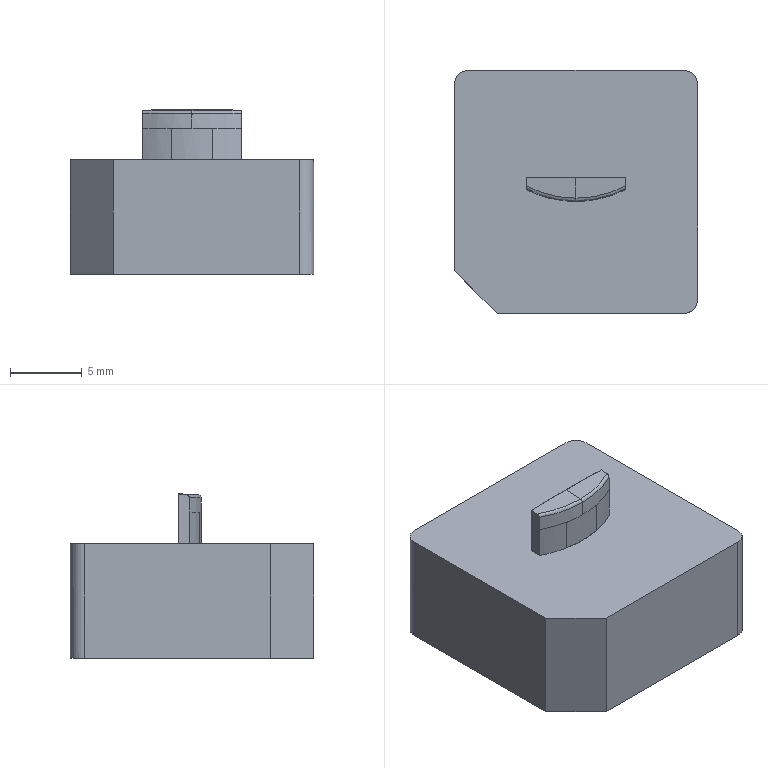NC program | PowerMill | posted with a generic post | part box 17 x 17 x 11.498 mm
Lines 1 to 991 of 31087:
%
O0001
N104 ( POWERMILL CB  : 2026004.0)
N105 ( POST VER      : 2026.0.0.5161)
N106 ( OPTION FILE   : FANUC)
N107 ( OUTPUT WORKPLANE : WORLD)
N108 (  )
N109 ( TOOL LIST )
N110 (-------------------------------------)
N111 ( NO. | ID      | DIA.| TIP RAD|LENGTH)
N112 (-------------------------------------)
N113 (    1|D10C_1_1 |10.0 |  0.0   |66.96 )
N114 (    2|D4C_1    | 4.0 |  0.0   | 59.0 )
N115 (    3|D10_1_1  |10.0 |  0.0   |66.64 )
N116 (    4|R1_1     | 2.0 |  1.0   | 57.0 )
N117 (   10|D3_1_1   | 3.0 |  0.0   |58.76 )
N118 (   13|TEXT_D4_1| 4.0 |  0.3   | 60.0 )
N119 (-------------------------------------)
N120 (  )
N121 ( NUMBER OF TOOLPATHS: 9.0 )
N122 ( ESTIMATED PROGRAM DURATION: 0 HOURS 2 MIN 53 SEC)
N123 (  )
N124 G00 G21 G80 G40 G17
N125 G90
N126 G54
N127 G53 Z0.0
N128 (---------------)
N129 ( START TOOLPATH : 精公开粗01-扫面平行-D10C )
N130 (---------------)
N131 ( TOOL NO.    :1 )
N132 ( TOOL TYPE   : ENDMILL)
N133 ( TOOL ID     : D10C_1_1)
N134 ( TOOL DIA    : 10.0 LENGTH 66.96)
N135 T1
N136 M6
N137 S8000 M03
N138 G00 G90 X0.0 Y0.0
N139 G43 Z10.2 H1
N140
N141 G05 P10000 R4
N142 X11.28 Y11.28
N143 Z1.128
N144 G01 Z-0.072 F6000.0
N145 X-11.28 F10000.0
N146 Y5.64
N147 X11.28
N148 Y0.0
N149 X-11.28
N150 Y-5.64
N151 X11.28
N152 Y-11.28
N153 X-11.28
N154 X-16.28
N155 G00 Z10.2
N156 G05 P0
N157 (---------------)
N158 ( END TOOLPATH : 精公开粗01-扫面平行-D10C )
N159 (---------------)
N160 ( START TOOLPATH : 精公开粗01-外形偏置-D10C )
N161 (---------------)
N162 G00 X0.0 Y0.0 Z9.878
N163 G05 P10000 R4
N164 X16.555 Y5.9194
N165 Z0.7016
N166 G01 Z-0.4984 F6000.0
N167 X16.0275 F10000.0
N168 G03 X11.28 Y1.1719 I0.0 J-4.7475
N169 G01 Y-10.28
N170 G02 X10.28 Y-11.28 I-1.0 J0.0
N171 G01 X-10.28
N172 G02 X-11.28 Y-10.28 I0.0 J1.0
N173 G01 Y10.28
N174 G02 X-10.28 Y11.28 I1.0 J0.0
N175 G01 X10.28
N176 G02 X11.28 Y10.28 I0.0 J-1.0
N177 G01 Y1.1719
N178 X8.7307 Y1.1601
N179 X8.7343 Y0.3867
N180 X8.7011 Y-0.3867
N181 X8.5538 Y-1.1601
N182 X8.2859 Y-1.9336
N183 X8.121 Y-2.2752
N184 X7.8634 Y-2.707
N185 X7.3476 Y-3.3716
N186 X6.5741 Y-4.0652
N187 X6.299 Y-4.2538
N188 X5.8007 Y-4.5354
N189 X4.6946 Y-5.0273
N190 X3.4804 Y-5.4313
N191 X2.707 Y-5.6154
N192 X1.6745 Y-5.8007
N193 X0.3867 Y-5.9046
N194 X-0.3867
N195 X-1.6743 Y-5.8007
N196 X-2.707 Y-5.6173
N197 X-3.4804 Y-5.4312
N198 X-4.2538 Y-5.1896
N199 X-4.6933 Y-5.0273
N200 X-5.8007 Y-4.5354
N201 X-6.3008 Y-4.2538
N202 X-6.5741 Y-4.0652
N203 X-7.2448 Y-3.4804
N204 X-7.8635 Y-2.707
N205 X-8.121 Y-2.2752
N206 X-8.2861 Y-1.9336
N207 X-8.5541 Y-1.1601
N208 X-8.6996 Y-0.3867
N209 X-8.7343 Y0.3867
N210 X-8.7307 Y1.1601
N211 X-8.6458 Y1.9336
N212 X-8.441 Y2.707
N213 X-8.121 Y3.442
N214 X-7.5905 Y4.2538
N215 X-7.3476 Y4.5389
N216 X-6.836 Y5.0273
N217 X-6.5741 Y5.232
N218 X-5.8007 Y5.7023
N219 X-5.0273 Y6.0126
N220 X-4.2538 Y6.1915
N221 X-3.4804 Y6.2524
N222 X3.4804
N223 X4.2538 Y6.1916
N224 X5.0273 Y6.0126
N225 X5.8007 Y5.7023
N226 X6.5741 Y5.232
N227 X6.836 Y5.0273
N228 X7.3476 Y4.5389
N229 X7.5906 Y4.2538
N230 X8.1004 Y3.4804
N231 X8.441 Y2.707
N232 X8.6459 Y1.9336
N233 X8.7307 Y1.1601
N234 X11.28 Y1.1719
N235 G00 Z3.3251
N236 G01 X16.555 Y5.9194
N237 G00 Z0.3251
N238 G01 Z-0.8749 F6000.0
N239 X16.0275 F10000.0
N240 G03 X11.28 Y1.1719 I0.0 J-4.7475
N241 G01 Y-10.28
N242 G02 X10.28 Y-11.28 I-1.0 J0.0
N243 G01 X-10.28
N244 G02 X-11.28 Y-10.28 I0.0 J1.0
N245 G01 Y10.28
N246 G02 X-10.28 Y11.28 I1.0 J0.0
N247 G01 X10.28
N248 G02 X11.28 Y10.28 I0.0 J-1.0
N249 G01 Y1.1719
N250 X8.7307 Y1.1601
N251 X8.7343 Y0.3867
N252 X8.7039 Y-0.3867
N253 X8.5619 Y-1.1601
N254 X8.2933 Y-1.9336
N255 X8.121 Y-2.2924
N256 X7.8768 Y-2.707
N257 X7.3476 Y-3.3893
N258 X6.5741 Y-4.0825
N259 X6.3254 Y-4.2538
N260 X5.8007 Y-4.5529
N261 X5.0273 Y-4.9088
N262 X4.2538 Y-5.2056
N263 X3.4804 Y-5.4458
N264 X2.707 Y-5.6321
N265 X1.7506 Y-5.8007
N266 X1.1601 Y-5.8702
N267 X0.3867 Y-5.9153
N268 X-0.3867 Y-5.9151
N269 X-1.1601 Y-5.872
N270 X-1.9336 Y-5.7768
N271 X-2.707 Y-5.6347
N272 X-3.4804 Y-5.4449
N273 X-4.2538 Y-5.2056
N274 X-4.7261 Y-5.0273
N275 X-5.8007 Y-4.5528
N276 X-6.3254 Y-4.2538
N277 X-6.5741 Y-4.0825
N278 X-7.2621 Y-3.4804
N279 X-7.8768 Y-2.707
N280 X-8.121 Y-2.2924
N281 X-8.2934 Y-1.9336
N282 X-8.5604 Y-1.1601
N283 X-8.7037 Y-0.3867
N284 X-8.7343 Y0.3867
N285 X-8.7308 Y1.1601
N286 X-8.6458 Y1.9336
N287 X-8.441 Y2.707
N288 X-8.121 Y3.442
N289 X-7.5906 Y4.2538
N290 X-7.3476 Y4.5389
N291 X-6.836 Y5.0273
N292 X-6.5741 Y5.232
N293 X-5.8007 Y5.7023
N294 X-5.0273 Y6.0126
N295 X-4.2538 Y6.1916
N296 X-3.4804 Y6.2524
N297 X3.4804
N298 X4.2538 Y6.1916
N299 X5.0273 Y6.0126
N300 X5.8007 Y5.7023
N301 X6.5741 Y5.232
N302 X6.836 Y5.0273
N303 X7.3476 Y4.5389
N304 X7.5906 Y4.2538
N305 X8.1004 Y3.4804
N306 X8.441 Y2.707
N307 X8.6459 Y1.9336
N308 X8.7307 Y1.1601
N309 X11.28 Y1.1719
N310 G00 Z2.9487
N311 G01 X16.555 Y5.9194
N312 G00 Z-0.0513
N313 G01 Z-1.2513 F6000.0
N314 X16.0275 F10000.0
N315 G03 X11.28 Y1.1719 I0.0 J-4.7475
N316 G01 Y-10.28
N317 G02 X10.28 Y-11.28 I-1.0 J0.0
N318 G01 X-10.28
N319 G02 X-11.28 Y-10.28 I0.0 J1.0
N320 G01 Y10.28
N321 G02 X-10.28 Y11.28 I1.0 J0.0
N322 G01 X10.28
N323 G02 X11.28 Y10.28 I0.0 J-1.0
N324 G01 Y1.1719
N325 X8.7307 Y1.1601
N326 X8.7343 Y0.3867
N327 X8.7054 Y-0.3867
N328 X8.5658 Y-1.1601
N329 X8.3003 Y-1.9336
N330 X8.121 Y-2.3071
N331 X7.8863 Y-2.707
N332 X7.3476 Y-3.4041
N333 X6.5741 Y-4.0972
N334 X6.348 Y-4.2538
N335 X5.8007 Y-4.5676
N336 X5.0273 Y-4.9231
N337 X4.2538 Y-5.2196
N338 X3.4804 Y-5.4604
N339 X2.707 Y-5.6475
N340 X1.8669 Y-5.8007
N341 X1.1601 Y-5.8843
N342 X0.3867 Y-5.9295
N343 X-0.3867 Y-5.9271
N344 X-1.1601 Y-5.8852
N345 X-1.9336 Y-5.7905
N346 X-2.707 Y-5.6483
N347 X-3.4804 Y-5.4586
N348 X-4.2538 Y-5.2195
N349 X-4.7621 Y-5.0273
N350 X-5.8007 Y-4.5675
N351 X-6.348 Y-4.2538
N352 X-6.5741 Y-4.0972
N353 X-7.2761 Y-3.4804
N354 X-7.8863 Y-2.707
N355 X-8.121 Y-2.3071
N356 X-8.3002 Y-1.9336
N357 X-8.5658 Y-1.1601
N358 X-8.7054 Y-0.3867
N359 X-8.7343 Y0.3867
N360 X-8.7308 Y1.1601
N361 X-8.6458 Y1.9336
N362 X-8.441 Y2.707
N363 X-8.121 Y3.442
N364 X-7.5906 Y4.2538
N365 X-7.3476 Y4.5389
N366 X-6.836 Y5.0273
N367 X-6.5741 Y5.232
N368 X-5.8007 Y5.7023
N369 X-5.0273 Y6.0126
N370 X-4.2538 Y6.1916
N371 X-3.4804 Y6.2524
N372 X3.4804
N373 X4.2538 Y6.1916
N374 X5.0273 Y6.0126
N375 X5.8007 Y5.7023
N376 X6.5741 Y5.232
N377 X6.836 Y5.0273
N378 X7.3476 Y4.5389
N379 X7.5906 Y4.2538
N380 X8.1004 Y3.4804
N381 X8.441 Y2.707
N382 X8.6459 Y1.9336
N383 X8.7307 Y1.1601
N384 X11.28 Y1.1719
N385 G00 Z2.5722
N386 G01 X16.555 Y5.9194
N387 G00 Z-0.4278
N388 G01 Z-1.6278 F6000.0
N389 X16.0275 F10000.0
N390 G03 X11.28 Y1.1719 I0.0 J-4.7475
N391 G01 Y-10.28
N392 G02 X10.28 Y-11.28 I-1.0 J0.0
N393 G01 X-10.28
N394 G02 X-11.28 Y-10.28 I0.0 J1.0
N395 G01 Y10.28
N396 G02 X-10.28 Y11.28 I1.0 J0.0
N397 G01 X10.28
N398 G02 X11.28 Y10.28 I0.0 J-1.0
N399 G01 Y1.1719
N400 X8.7307 Y1.1601
N401 X8.7343 Y0.3867
N402 X8.7063 Y-0.3867
N403 X8.568 Y-1.1601
N404 X8.3041 Y-1.9336
N405 X8.121 Y-2.3162
N406 X7.8922 Y-2.707
N407 X7.3476 Y-3.413
N408 X6.5741 Y-4.1062
N409 X6.3618 Y-4.2538
N410 X5.8007 Y-4.5765
N411 X5.0273 Y-4.9321
N412 X4.2538 Y-5.2286
N413 X3.4804 Y-5.4701
N414 X2.707 Y-5.6563
N415 X1.9271 Y-5.8007
N416 X1.1601 Y-5.8939
N417 X0.3867 Y-5.9396
N418 X-0.3867 Y-5.94
N419 X-1.1601 Y-5.8942
N420 X-1.9283 Y-5.8007
N421 X-2.707 Y-5.6574
N422 X-3.4804 Y-5.4701
N423 X-4.2538 Y-5.2284
N424 X-5.0273 Y-4.932
N425 X-5.8007 Y-4.5765
N426 X-6.3618 Y-4.2538
N427 X-6.5741 Y-4.1062
N428 X-7.2848 Y-3.4804
N429 X-7.8922 Y-2.707
N430 X-8.121 Y-2.3162
N431 X-8.3041 Y-1.9336
N432 X-8.5681 Y-1.1601
N433 X-8.7063 Y-0.3867
N434 X-8.7343 Y0.3867
N435 X-8.7308 Y1.1601
N436 X-8.6458 Y1.9336
N437 X-8.441 Y2.707
N438 X-8.121 Y3.442
N439 X-7.5906 Y4.2538
N440 X-7.3476 Y4.5389
N441 X-6.836 Y5.0273
N442 X-6.5741 Y5.232
N443 X-5.8007 Y5.7023
N444 X-5.0273 Y6.0126
N445 X-4.2538 Y6.1916
N446 X-3.4804 Y6.2524
N447 X3.4804
N448 X4.2538 Y6.1916
N449 X5.0273 Y6.0126
N450 X5.8007 Y5.7023
N451 X6.5741 Y5.232
N452 X6.836 Y5.0273
N453 X7.3476 Y4.5389
N454 X7.5906 Y4.2538
N455 X8.1004 Y3.4804
N456 X8.4411 Y2.707
N457 X8.6459 Y1.9336
N458 X8.7307 Y1.1601
N459 X11.28 Y1.1719
N460 G00 Z2.1958
N461 G01 X16.555 Y5.9194
N462 G00 Z-0.8042
N463 G01 Z-2.0042 F6000.0
N464 X16.0275 F10000.0
N465 G03 X11.28 Y1.1719 I0.0 J-4.7475
N466 G01 Y-10.28
N467 G02 X10.28 Y-11.28 I-1.0 J0.0
N468 G01 X-10.28
N469 G02 X-11.28 Y-10.28 I0.0 J1.0
N470 G01 Y10.28
N471 G02 X-10.28 Y11.28 I1.0 J0.0
N472 G01 X10.28
N473 G02 X11.28 Y10.28 I0.0 J-1.0
N474 G01 Y1.1719
N475 X8.7307 Y1.1601
N476 X8.7343 Y0.3867
N477 X8.7063 Y-0.3867
N478 X8.568 Y-1.1601
N479 X8.3041 Y-1.9336
N480 X8.121 Y-2.3162
N481 X7.8922 Y-2.707
N482 X7.3476 Y-3.413
N483 X6.5741 Y-4.1062
N484 X6.3618 Y-4.2538
N485 X5.8007 Y-4.5766
N486 X5.0273 Y-4.9322
N487 X4.2538 Y-5.2286
N488 X3.4804 Y-5.4701
N489 X2.707 Y-5.6582
N490 X1.9272 Y-5.8007
N491 X1.1601 Y-5.8939
N492 X0.3867 Y-5.9396
N493 X-0.3867 Y-5.9401
N494 X-1.1601 Y-5.8942
N495 X-1.9283 Y-5.8007
N496 X-2.707 Y-5.6574
N497 X-3.4804 Y-5.4701
N498 X-4.2538 Y-5.2285
N499 X-4.7873 Y-5.0273
N500 X-4.8423 Y-5.0028
N501 X-5.0273 Y-4.9319
N502 X-5.7958 Y-4.5787
N503 X-5.8007 Y-4.5766
N504 X-6.3618 Y-4.2538
N505 X-6.5741 Y-4.1062
N506 X-7.2848 Y-3.4804
N507 X-7.8922 Y-2.707
N508 X-8.121 Y-2.3162
N509 X-8.3042 Y-1.9336
N510 X-8.5681 Y-1.1601
N511 X-8.7064 Y-0.3867
N512 X-8.7343 Y0.3867
N513 X-8.7308 Y1.1601
N514 X-8.6458 Y1.9336
N515 X-8.441 Y2.707
N516 X-8.121 Y3.442
N517 X-7.5906 Y4.2538
N518 X-7.3476 Y4.5389
N519 X-6.836 Y5.0273
N520 X-6.5741 Y5.232
N521 X-5.8007 Y5.7023
N522 X-5.0273 Y6.0127
N523 X-4.2538 Y6.1916
N524 X-3.4804 Y6.2524
N525 X3.4804
N526 X4.2538 Y6.1916
N527 X5.0273 Y6.0127
N528 X5.8007 Y5.7023
N529 X6.5741 Y5.232
N530 X6.836 Y5.0273
N531 X7.3476 Y4.5389
N532 X7.5907 Y4.2538
N533 X8.1005 Y3.4804
N534 X8.4411 Y2.707
N535 X8.6459 Y1.9336
N536 X8.7307 Y1.1601
N537 X11.28 Y1.1719
N538 G00 Z1.8193
N539 G01 X16.555 Y5.9194
N540 G00 Z-1.1807
N541 G01 Z-2.3807 F6000.0
N542 X16.0275 F10000.0
N543 G03 X11.28 Y1.1719 I0.0 J-4.7475
N544 G01 Y-10.28
N545 G02 X10.28 Y-11.28 I-1.0 J0.0
N546 G01 X-10.28
N547 G02 X-11.28 Y-10.28 I0.0 J1.0
N548 G01 Y10.28
N549 G02 X-10.28 Y11.28 I1.0 J0.0
N550 G01 X10.28
N551 G02 X11.28 Y10.28 I0.0 J-1.0
N552 G01 Y1.1719
N553 X8.7307 Y1.1601
N554 X8.7343 Y0.3867
N555 X8.7064 Y-0.3867
N556 X8.5681 Y-1.1601
N557 X8.3041 Y-1.9336
N558 X8.121 Y-2.3162
N559 X7.8922 Y-2.707
N560 X7.3476 Y-3.413
N561 X6.5741 Y-4.1062
N562 X6.3618 Y-4.2538
N563 X5.8007 Y-4.5766
N564 X5.0273 Y-4.9322
N565 X4.2538 Y-5.2286
N566 X3.4804 Y-5.4701
N567 X2.707 Y-5.6589
N568 X1.9272 Y-5.8007
N569 X1.1601 Y-5.894
N570 X0.3867 Y-5.9396
N571 X-0.3867 Y-5.9401
N572 X-1.1601 Y-5.8942
N573 X-1.9283 Y-5.8007
N574 X-2.707 Y-5.6574
N575 X-3.4804 Y-5.4701
N576 X-4.2538 Y-5.2285
N577 X-4.7891 Y-5.0273
N578 X-4.8553 Y-4.9978
N579 X-5.0272 Y-4.9319
N580 X-5.7904 Y-4.5812
N581 X-5.8007 Y-4.5766
N582 X-6.3618 Y-4.2538
N583 X-6.5741 Y-4.1062
N584 X-7.2848 Y-3.4804
N585 X-7.8922 Y-2.707
N586 X-8.121 Y-2.3162
N587 X-8.3042 Y-1.9336
N588 X-8.5681 Y-1.1601
N589 X-8.7064 Y-0.3867
N590 X-8.7343 Y0.3867
N591 X-8.7308 Y1.1601
N592 X-8.6459 Y1.9336
N593 X-8.441 Y2.707
N594 X-8.121 Y3.442
N595 X-7.5906 Y4.2538
N596 X-7.3476 Y4.5389
N597 X-6.836 Y5.0273
N598 X-6.5741 Y5.232
N599 X-5.8007 Y5.7024
N600 X-5.0273 Y6.0127
N601 X-4.2538 Y6.1916
N602 X-3.4804 Y6.2524
N603 X3.4804
N604 X4.2538 Y6.1916
N605 X5.0273 Y6.0127
N606 X5.8007 Y5.7024
N607 X6.5741 Y5.232
N608 X6.836 Y5.0273
N609 X7.3476 Y4.5389
N610 X7.5907 Y4.2538
N611 X8.1005 Y3.4804
N612 X8.4411 Y2.707
N613 X8.6459 Y1.9336
N614 X8.7307 Y1.1601
N615 X11.28 Y1.1719
N616 G00 Z1.4429
N617 G01 X16.555 Y5.9194
N618 G00 Z-1.5571
N619 G01 Z-2.7571 F6000.0
N620 X16.0275 F10000.0
N621 G03 X11.28 Y1.1719 I0.0 J-4.7475
N622 G01 Y-10.28
N623 G02 X10.28 Y-11.28 I-1.0 J0.0
N624 G01 X-10.28
N625 G02 X-11.28 Y-10.28 I0.0 J1.0
N626 G01 Y10.28
N627 G02 X-10.28 Y11.28 I1.0 J0.0
N628 G01 X10.28
N629 G02 X11.28 Y10.28 I0.0 J-1.0
N630 G01 Y1.1719
N631 X8.7307 Y1.1601
N632 X8.7343 Y0.3867
N633 X8.7064 Y-0.3867
N634 X8.5681 Y-1.1601
N635 X8.3041 Y-1.9336
N636 X8.121 Y-2.3162
N637 X7.8922 Y-2.707
N638 X7.3476 Y-3.413
N639 X6.5741 Y-4.1062
N640 X6.3618 Y-4.2538
N641 X5.8007 Y-4.5766
N642 X5.0273 Y-4.9322
N643 X4.2538 Y-5.2287
N644 X3.4804 Y-5.4701
N645 X2.707 Y-5.6595
N646 X1.9272 Y-5.8007
N647 X1.1601 Y-5.894
N648 X0.3867 Y-5.9396
N649 X-0.3867 Y-5.9401
N650 X-1.1601 Y-5.8943
N651 X-1.9283 Y-5.8007
N652 X-2.707 Y-5.6575
N653 X-3.4804 Y-5.4701
N654 X-4.2538 Y-5.2285
N655 X-4.7908 Y-5.0273
N656 X-4.8678 Y-4.9929
N657 X-5.0272 Y-4.9318
N658 X-5.7844 Y-4.5839
N659 X-5.8007 Y-4.5766
N660 X-6.3619 Y-4.2538
N661 X-6.5741 Y-4.1062
N662 X-7.2848 Y-3.4804
N663 X-7.8922 Y-2.707
N664 X-8.121 Y-2.3162
N665 X-8.3042 Y-1.9336
N666 X-8.5681 Y-1.1601
N667 X-8.7064 Y-0.3867
N668 X-8.7343 Y0.3867
N669 X-8.7308 Y1.1601
N670 X-8.6459 Y1.9336
N671 X-8.4411 Y2.707
N672 X-8.121 Y3.442
N673 X-7.5906 Y4.2538
N674 X-7.3476 Y4.5389
N675 X-6.836 Y5.0273
N676 X-6.5741 Y5.232
N677 X-5.8007 Y5.7024
N678 X-5.0273 Y6.0127
N679 X-4.2538 Y6.1916
N680 X-3.4804 Y6.2524
N681 X3.4804 Y6.2525
N682 X4.2538 Y6.1916
N683 X5.0273 Y6.0127
N684 X5.8007 Y5.7024
N685 X6.5741 Y5.232
N686 X6.836 Y5.0273
N687 X7.3476 Y4.5389
N688 X7.5907 Y4.2538
N689 X8.1005 Y3.4804
N690 X8.4411 Y2.707
N691 X8.6459 Y1.9336
N692 X8.7307 Y1.1601
N693 X11.28 Y1.1719
N694 G00 Z1.0665
N695 G01 X16.555 Y5.9194
N696 G00 Z-1.9335
N697 G01 Z-3.1335 F6000.0
N698 X16.0275 F10000.0
N699 G03 X11.28 Y1.1719 I0.0 J-4.7475
N700 G01 Y-10.28
N701 G02 X10.28 Y-11.28 I-1.0 J0.0
N702 G01 X-10.28
N703 G02 X-11.28 Y-10.28 I0.0 J1.0
N704 G01 Y10.28
N705 G02 X-10.28 Y11.28 I1.0 J0.0
N706 G01 X10.28
N707 G02 X11.28 Y10.28 I0.0 J-1.0
N708 G01 Y1.1719
N709 X8.7308 Y1.1601
N710 X8.7343 Y0.3867
N711 X8.7064 Y-0.3867
N712 X8.5681 Y-1.1601
N713 X8.3041 Y-1.9336
N714 X8.121 Y-2.3162
N715 X7.8922 Y-2.707
N716 X7.3476 Y-3.4131
N717 X6.5741 Y-4.1063
N718 X6.3619 Y-4.2538
N719 X5.8007 Y-4.5766
N720 X5.0273 Y-4.9322
N721 X4.2538 Y-5.2287
N722 X3.4804 Y-5.4701
N723 X2.707 Y-5.6601
N724 X1.9272 Y-5.8007
N725 X1.1601 Y-5.894
N726 X0.3867 Y-5.9396
N727 X-0.3867 Y-5.9401
N728 X-1.1601 Y-5.8943
N729 X-1.9284 Y-5.8007
N730 X-2.707 Y-5.6575
N731 X-3.4804 Y-5.4701
N732 X-4.2538 Y-5.2285
N733 X-4.7925 Y-5.0273
N734 X-4.8796 Y-4.9884
N735 X-5.0272 Y-4.9318
N736 X-5.7777 Y-4.5869
N737 X-5.8007 Y-4.5766
N738 X-6.3619 Y-4.2538
N739 X-6.5741 Y-4.1063
N740 X-7.2848 Y-3.4804
N741 X-7.8922 Y-2.707
N742 X-8.121 Y-2.3162
N743 X-8.3042 Y-1.9336
N744 X-8.5681 Y-1.1601
N745 X-8.7064 Y-0.3867
N746 X-8.7343 Y0.3867
N747 X-8.7308 Y1.1601
N748 X-8.6459 Y1.9336
N749 X-8.4411 Y2.707
N750 X-8.121 Y3.442
N751 X-7.5906 Y4.2538
N752 X-7.3476 Y4.539
N753 X-6.836 Y5.0273
N754 X-6.5741 Y5.232
N755 X-5.8007 Y5.7024
N756 X-5.0273 Y6.0127
N757 X-4.2538 Y6.1916
N758 X-3.4804 Y6.2524
N759 X3.4804 Y6.2525
N760 X4.2538 Y6.1916
N761 X5.0273 Y6.0127
N762 X5.8007 Y5.7024
N763 X6.5741 Y5.232
N764 X6.836 Y5.0273
N765 X7.3476 Y4.539
N766 X7.5907 Y4.2538
N767 X8.1005 Y3.4804
N768 X8.4411 Y2.707
N769 X8.6459 Y1.9336
N770 X8.7308 Y1.1601
N771 X11.28 Y1.1719
N772 G00 Z0.69
N773 G01 X16.555 Y5.9194
N774 G00 Z-2.31
N775 G01 Z-3.51 F6000.0
N776 X16.0275 F10000.0
N777 G03 X11.28 Y1.1719 I0.0 J-4.7475
N778 G01 Y-10.28
N779 G02 X10.28 Y-11.28 I-1.0 J0.0
N780 G01 X-10.28
N781 G02 X-11.28 Y-10.28 I0.0 J1.0
N782 G01 Y10.28
N783 G02 X-10.28 Y11.28 I1.0 J0.0
N784 G01 X10.28
N785 G02 X11.28 Y10.28 I0.0 J-1.0
N786 G01 Y1.1719
N787 X8.7308 Y1.1601
N788 X8.7343 Y0.3867
N789 X8.7064 Y-0.3867
N790 X8.5681 Y-1.1601
N791 X8.3042 Y-1.9336
N792 X8.121 Y-2.3163
N793 X7.8923 Y-2.707
N794 X7.3476 Y-3.4131
N795 X6.5741 Y-4.1063
N796 X6.3619 Y-4.2538
N797 X5.8007 Y-4.5766
N798 X5.0273 Y-4.9322
N799 X4.2538 Y-5.2287
N800 X3.4804 Y-5.4702
N801 X2.707 Y-5.6605
N802 X1.9273 Y-5.8007
N803 X1.1601 Y-5.894
N804 X0.3867 Y-5.9397
N805 X-0.3867 Y-5.9401
N806 X-1.1601 Y-5.8943
N807 X-1.9284 Y-5.8007
N808 X-2.707 Y-5.6575
N809 X-3.4804 Y-5.4702
N810 X-4.2538 Y-5.2285
N811 X-4.7935 Y-5.0273
N812 X-4.8867 Y-4.9856
N813 X-5.0272 Y-4.9317
N814 X-5.7709 Y-4.59
N815 X-5.8007 Y-4.5766
N816 X-6.3619 Y-4.2538
N817 X-6.5741 Y-4.1063
N818 X-7.2848 Y-3.4804
N819 X-7.8922 Y-2.707
N820 X-8.121 Y-2.3163
N821 X-8.3042 Y-1.9336
N822 X-8.5682 Y-1.1601
N823 X-8.7064 Y-0.3867
N824 X-8.7343 Y0.3867
N825 X-8.7308 Y1.1601
N826 X-8.6459 Y1.9336
N827 X-8.4411 Y2.707
N828 X-8.121 Y3.4421
N829 X-7.5906 Y4.2538
N830 X-7.3476 Y4.539
N831 X-6.836 Y5.0273
N832 X-6.5741 Y5.232
N833 X-5.8007 Y5.7024
N834 X-5.0273 Y6.0127
N835 X-4.2538 Y6.1916
N836 X-3.4804 Y6.2524
N837 X3.4804 Y6.2525
N838 X4.2538 Y6.1917
N839 X5.0273 Y6.0127
N840 X5.8007 Y5.7024
N841 X6.5741 Y5.232
N842 X6.836 Y5.0273
N843 X7.3476 Y4.539
N844 X7.5907 Y4.2538
N845 X8.1005 Y3.4804
N846 X8.4411 Y2.707
N847 X8.6459 Y1.9336
N848 X8.7308 Y1.1601
N849 X11.28 Y1.1719
N850 G00 Z9.878
N851 G05 P0
N852 (---------------)
N853 ( END TOOLPATH : 精公开粗01-外形偏置-D10C )
N854 (---------------)
N855 ( START TOOLPATH : 精公开粗01-基准台等高-D10C )
N856 (---------------)
N857 G00 X0.0 Y0.0 Z9.7979
N858 G05 P10000 R4
N859 X11.719 Y-18.8045
N860 Z-2.6881
N861 G01 Z-3.8881 F6000.0
N862 G03 X9.7172 Y-13.1483 I-1.0009 J2.8281 F10000.0
N863 G01 X9.2811 Y-13.3026
N864 X8.5077 Y-13.4819
N865 X7.7343 Y-13.5646
N866 X-5.414 Y-13.57
N867 X-6.1874 Y-13.5232
N868 X-6.9608 Y-13.355
N869 X-7.7343 Y-13.0511
N870 X-8.5077 Y-12.5815
N871 X-8.7696 Y-12.3748
N872 X-9.2811 Y-11.8889
N873 X-11.8889 Y-9.2811
N874 X-12.3748 Y-8.7696
N875 X-12.5815 Y-8.5077
N876 X-13.0511 Y-7.7343
N877 X-13.355 Y-6.9608
N878 X-13.5232 Y-6.1874
N879 X-13.57 Y-5.414
N880 X-13.5646 Y7.7343
N881 X-13.4819 Y8.5077
N882 X-13.3026 Y9.2811
N883 X-13.0024 Y10.0545
N884 X-12.5746 Y10.828
N885 X-12.3748 Y11.1166
N886 X-11.9732 Y11.6014
N887 X-11.6014 Y11.9732
N888 X-11.1166 Y12.3748
N889 X-10.828 Y12.5747
N890 X-10.0545 Y13.0024
N891 X-9.2811 Y13.3026
N892 X-8.5077 Y13.4819
N893 X-7.7343 Y13.5645
N894 X7.7343
N895 X8.5077 Y13.4819
N896 X9.2811 Y13.3026
N897 X10.0545 Y13.0024
N898 X10.828 Y12.5747
N899 X11.1167 Y12.3748
N900 X11.6014 Y11.9732
N901 X11.9732 Y11.6014
N902 X12.3748 Y11.1167
N903 X12.5747 Y10.828
N904 X13.0024 Y10.0545
N905 X13.3026 Y9.2811
N906 X13.4819 Y8.5077
N907 X13.5646 Y7.7343
N908 Y-7.7343
N909 X13.4818 Y-8.5077
N910 X13.3026 Y-9.2811
N911 X13.0024 Y-10.0545
N912 X12.5747 Y-10.828
N913 X12.3748 Y-11.1166
N914 X11.9732 Y-11.6014
N915 X11.6014 Y-11.9732
N916 X11.1166 Y-12.3748
N917 X10.828 Y-12.5746
N918 X10.0545 Y-13.0024
N919 X9.7172 Y-13.1483
N920 X9.2811 Y-13.3026 Z-3.89
N921 X8.5077 Y-13.4819 Z-3.8931
N922 X7.7343 Y-13.5646 Z-3.8963
N923 X-5.414 Y-13.57 Z-3.949
N924 X-6.1996 Y-13.5215 Z-3.9521
N925 X-6.9698 Y-13.3523 Z-3.9553
N926 X-7.7469 Y-13.0449 Z-3.9587
N927 X-8.5119 Y-12.5784 Z-3.9622
N928 X-8.7696 Y-12.3748 Z-3.9636
N929 X-9.2811 Y-11.8889 Z-3.9664
N930 X-11.8967 Y-9.2733 Z-3.9812
N931 X-12.3782 Y-8.7656 Z-3.984
N932 X-12.5815 Y-8.5077 Z-3.9853
N933 X-13.0511 Y-7.7343 Z-3.989
N934 X-13.355 Y-6.9608 Z-3.9923
N935 X-13.5232 Y-6.1874 Z-3.9955
N936 X-13.57 Y-5.414 Z-3.9986
N937 X-13.5646 Y7.7343 Z-4.0513
N938 X-13.48 Y8.5199 Z-4.0545
N939 X-13.3005 Y9.288 Z-4.0576
N940 X-12.9968 Y10.0671 Z-4.061
N941 X-12.5717 Y10.8326 Z-4.0645
N942 X-12.3748 Y11.1166 Z-4.0659
N943 X-11.9677 Y11.6075 Z-4.0685
N944 X-11.6014 Y11.9732 Z-4.0705
N945 X-11.1166 Y12.3749 Z-4.0731
N946 X-10.828 Y12.5747 Z-4.0745
N947 X-10.0546 Y13.0024 Z-4.078
N948 X-9.2811 Y13.3026 Z-4.0813
N949 X-8.5077 Y13.4819 Z-4.0845
N950 X-7.7343 Y13.5646 Z-4.0876
N951 X7.7343 Z-4.1497
N952 X8.5199 Y13.48 Z-4.1528
N953 X9.288 Y13.3005 Z-4.156
N954 X10.0671 Y12.9968 Z-4.1594
N955 X10.8326 Y12.5717 Z-4.1629
N956 X11.1167 Y12.3748 Z-4.1643
N957 X11.6075 Y11.9677 Z-4.1668
N958 X11.9732 Y11.6014 Z-4.1689
N959 X12.3748 Y11.1167 Z-4.1714
N960 X12.5747 Y10.828 Z-4.1728
N961 X13.0024 Y10.0545 Z-4.1764
N962 X13.3026 Y9.2811 Z-4.1797
N963 X13.4819 Y8.5077 Z-4.1829
N964 X13.5646 Y7.7343 Z-4.186
N965 Y-7.7343 Z-4.248
N966 X13.48 Y-8.5199 Z-4.2512
N967 X13.3005 Y-9.288 Z-4.2544
N968 X12.9968 Y-10.0671 Z-4.2577
N969 X12.5718 Y-10.8326 Z-4.2612
N970 X12.3749 Y-11.1166 Z-4.2626
N971 X11.9677 Y-11.6075 Z-4.2652
N972 X11.6014 Y-11.9732 Z-4.2672
N973 X11.1166 Y-12.3748 Z-4.2698
N974 X10.828 Y-12.5747 Z-4.2712
N975 X10.0545 Y-13.0024 Z-4.2747
N976 X9.7172 Y-13.1483 Z-4.2762
N977 X9.2811 Y-13.3026 Z-4.278
N978 X8.5077 Y-13.4819 Z-4.2812
N979 X7.7343 Y-13.5646 Z-4.2843
N980 X-5.414 Y-13.57 Z-4.3371
N981 X-6.1996 Y-13.5215 Z-4.3402
N982 X-6.9698 Y-13.3523 Z-4.3434
N983 X-7.7469 Y-13.0449 Z-4.3467
N984 X-8.5119 Y-12.5784 Z-4.3503
N985 X-8.7696 Y-12.3748 Z-4.3517
N986 X-9.2811 Y-11.8889 Z-4.3545
N987 X-11.8967 Y-9.2733 Z-4.3693
N988 X-12.3782 Y-8.7657 Z-4.3721
N989 X-12.5815 Y-8.5077 Z-4.3734
N990 X-13.0511 Y-7.7343 Z-4.3771
N991 X-13.355 Y-6.9608 Z-4.3804
N992 X-13.5232 Y-6.1874 Z-4.3836
N993 X-13.57 Y-5.414 Z-4.3867
N994 X-13.5646 Y7.7343 Z-4.4394
N995 X-13.48 Y8.5199 Z-4.4426
N996 X-13.3005 Y9.288 Z-4.4457
N997 X-12.9968 Y10.0671 Z-4.4491
N998 X-12.5717 Y10.8326 Z-4.4526
N999 X-12.3748 Y11.1166 Z-4.454
N1000 X-11.9677 Y11.6075 Z-4.4566
N1001 X-11.6014 Y11.9732 Z-4.4586
N1002 X-11.1166 Y12.3749 Z-4.4612
N1003 X-10.828 Y12.5747 Z-4.4626
N1004 X-10.0546 Y13.0024 Z-4.4661
N1005 X-9.2811 Y13.3026 Z-4.4694
N1006 X-8.5077 Y13.4819 Z-4.4726
N1007 X-7.7343 Y13.5646 Z-4.4757
N1008 X7.7343 Z-4.5378
N1009 X8.5199 Y13.48 Z-4.5409
N1010 X9.288 Y13.3005 Z-4.5441
N1011 X10.0671 Y12.9968 Z-4.5475
N1012 X10.8326 Y12.5718 Z-4.551
N1013 X11.1167 Y12.3748 Z-4.5523
N1014 X11.6075 Y11.9677 Z-4.5549
N1015 X11.9732 Y11.6014 Z-4.557
N1016 X12.3748 Y11.1167 Z-4.5595
N1017 X12.5747 Y10.828 Z-4.5609
N1018 X13.0024 Y10.0545 Z-4.5645
N1019 X13.3026 Y9.2811 Z-4.5678
N1020 X13.4819 Y8.5077 Z-4.571
N1021 X13.5646 Y7.7343 Z-4.5741
N1022 Y-7.7343 Z-4.6361
N1023 X13.48 Y-8.5199 Z-4.6393
N1024 X13.3005 Y-9.288 Z-4.6425
N1025 X12.9968 Y-10.0671 Z-4.6458
N1026 X12.5718 Y-10.8326 Z-4.6493
N1027 X12.3749 Y-11.1166 Z-4.6507
N1028 X11.9677 Y-11.6075 Z-4.6533
N1029 X11.6014 Y-11.9732 Z-4.6553
N1030 X11.1166 Y-12.3748 Z-4.6579
N1031 X10.828 Y-12.5747 Z-4.6593
N1032 X10.0545 Y-13.0024 Z-4.6628
N1033 X9.7172 Y-13.1483 Z-4.6643
N1034 X9.2811 Y-13.3026 Z-4.6661
N1035 X8.5077 Y-13.4819 Z-4.6693
N1036 X7.7343 Y-13.5646 Z-4.6724
N1037 X-5.414 Y-13.57 Z-4.7252
N1038 X-6.1996 Y-13.5215 Z-4.7283
N1039 X-6.9698 Y-13.3523 Z-4.7315
N1040 X-7.7469 Y-13.0449 Z-4.7348
N1041 X-8.5119 Y-12.5784 Z-4.7384
N1042 X-8.7696 Y-12.3748 Z-4.7398
N1043 X-9.2811 Y-11.8889 Z-4.7426
N1044 X-11.8967 Y-9.2733 Z-4.7574
N1045 X-12.3782 Y-8.7657 Z-4.7602
N1046 X-12.5815 Y-8.5077 Z-4.7615
N1047 X-13.0511 Y-7.7343 Z-4.7652
N1048 X-13.355 Y-6.9608 Z-4.7685
N1049 X-13.5232 Y-6.1874 Z-4.7717
N1050 X-13.57 Y-5.414 Z-4.7748
N1051 X-13.5646 Y7.7343 Z-4.8275
N1052 X-13.48 Y8.5199 Z-4.8307
N1053 X-13.3005 Y9.288 Z-4.8338
N1054 X-12.9968 Y10.0671 Z-4.8372
N1055 X-12.5717 Y10.8326 Z-4.8407
N1056 X-12.3748 Y11.1166 Z-4.8421
N1057 X-11.9677 Y11.6075 Z-4.8446
N1058 X-11.6014 Y11.9732 Z-4.8467
N1059 X-11.1166 Y12.3749 Z-4.8492
N1060 X-10.828 Y12.5747 Z-4.8507
N1061 X-10.0546 Y13.0024 Z-4.8542
N1062 X-9.2811 Y13.3026 Z-4.8575
N1063 X-8.5077 Y13.4819 Z-4.8607
N1064 X-7.7343 Y13.5646 Z-4.8638
N1065 X7.7343 Z-4.9259
N1066 X8.5199 Y13.48 Z-4.929
N1067 X9.288 Y13.3005 Z-4.9322
N1068 X10.0671 Y12.9968 Z-4.9355
N1069 X10.8326 Y12.5718 Z-4.9391
N1070 X11.1167 Y12.3748 Z-4.9404
N1071 X11.6075 Y11.9677 Z-4.943
N1072 X11.9732 Y11.6014 Z-4.9451
N1073 X12.3748 Y11.1167 Z-4.9476
N1074 X12.5747 Y10.828 Z-4.949
N1075 X13.0024 Y10.0545 Z-4.9526
N1076 X13.3026 Y9.2811 Z-4.9559
N1077 X13.4819 Y8.5077 Z-4.9591
N1078 X13.5646 Y7.7343 Z-4.9622
N1079 Y-7.7343 Z-5.0242
N1080 X13.48 Y-8.5199 Z-5.0274
N1081 X13.3005 Y-9.288 Z-5.0305
N1082 X12.9968 Y-10.0671 Z-5.0339
N1083 X12.5718 Y-10.8326 Z-5.0374
N1084 X12.3749 Y-11.1166 Z-5.0388
N1085 X11.9677 Y-11.6075 Z-5.0414
N1086 X11.6014 Y-11.9732 Z-5.0434
N1087 X11.1166 Y-12.3748 Z-5.046
N1088 X10.828 Y-12.5747 Z-5.0474